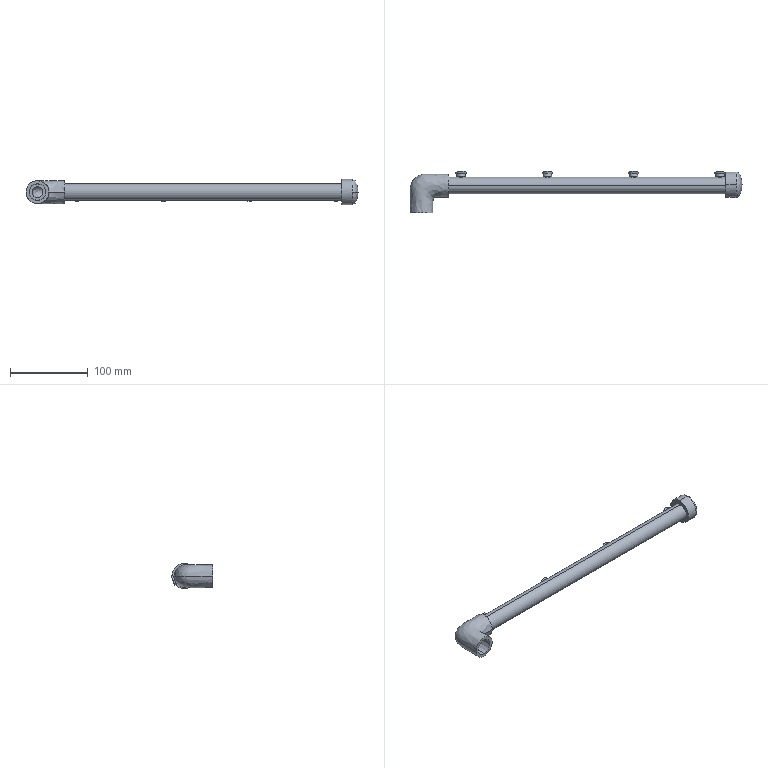Part | SolidWorks | 7 solids | 155 faces | box 426.966 x 53.25 x 32.766 mm | volume 119416 mm3 | cylinder 70 | plane 39 | cone 30 | torus 8 | spline 8 | commonest cylinder face diameters 8 x16 6.476 x8 10 x8 10.8 x8 10.935 x8 12.15 x8